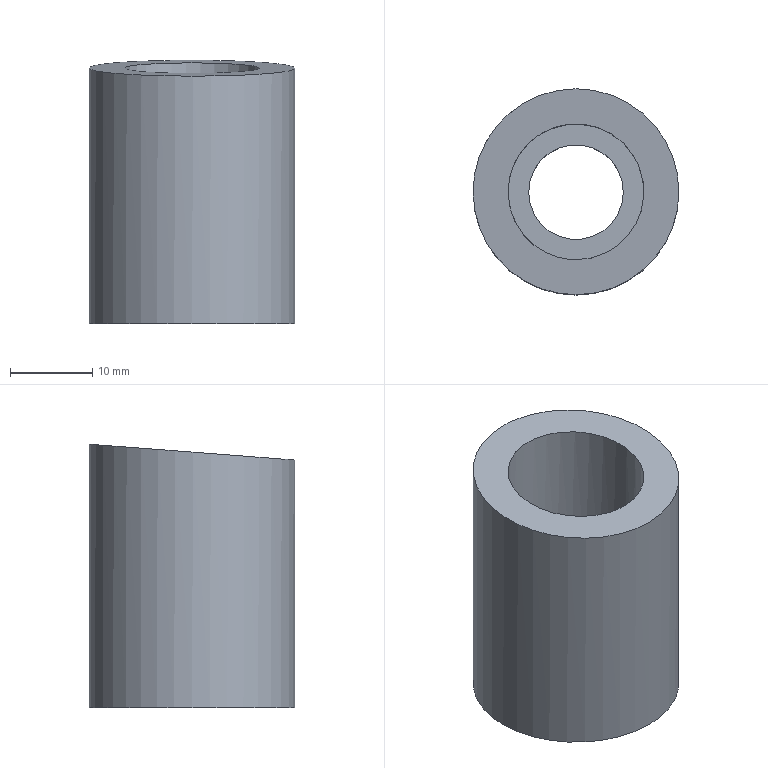Part | NX | features solid 2 | 1 solid | 6 faces | box 25 x 25 x 32.007 mm | volume 9815 mm3 | plane 3 | cylinder 3 | commonest cylinder face diameters 11.5 x1 16.5 x1 25 x1
STEP:
#1=CARTESIAN_POINT('',(-503.5,9.,-58.));
#2=VERTEX_POINT('',#1);
#3=CARTESIAN_POINT('',(-516.,9.,-58.));
#4=DIRECTION('',(0.,0.,1.));
#5=DIRECTION('',(1.,0.,0.));
#6=AXIS2_PLACEMENT_3D('',#3,#4,#5);
#7=CIRCLE('',#6,12.5);
#8=EDGE_CURVE('',#2,#2,#7,.T.);
#9=ORIENTED_EDGE('',*,*,#8,.F.);
#10=EDGE_LOOP('',(#9));
#11=FACE_BOUND('',#10,.T.);
#12=CARTESIAN_POINT('',(-510.25,9.,-58.));
#13=VERTEX_POINT('',#12);
#14=CARTESIAN_POINT('',(-516.,9.,-58.));
#15=DIRECTION('',(0.,0.,1.));
#16=DIRECTION('',(1.,0.,0.));
#17=AXIS2_PLACEMENT_3D('',#14,#15,#16);
#18=CIRCLE('',#17,5.75);
#19=EDGE_CURVE('',#13,#13,#18,.F.);
#20=ORIENTED_EDGE('',*,*,#19,.F.);
#21=EDGE_LOOP('',(#20));
#22=FACE_BOUND('',#21,.T.);
#23=CARTESIAN_POINT('',(-516.,9.,-58.));
#24=DIRECTION('',(0.,0.,1.));
#25=DIRECTION('',(1.,0.,0.));
#26=AXIS2_PLACEMENT_3D('',#23,#24,#25);
#27=PLANE('',#26);
#28=ADVANCED_FACE('',(#11,#22),#27,.F.);
#29=CARTESIAN_POINT('',(-507.75,9.,-46.955));
#30=VERTEX_POINT('',#29);
#31=CARTESIAN_POINT('',(-516.,9.,-46.955));
#32=DIRECTION('',(0.,0.,1.));
#33=DIRECTION('',(1.,0.,0.));
#34=AXIS2_PLACEMENT_3D('',#31,#32,#33);
#35=CIRCLE('',#34,8.25);
#36=EDGE_CURVE('',#30,#30,#35,.T.);
#37=ORIENTED_EDGE('',*,*,#36,.T.);
#38=EDGE_LOOP('',(#37));
#39=FACE_BOUND('',#38,.T.);
#40=CARTESIAN_POINT('',(-510.25,9.,-46.955));
#41=VERTEX_POINT('',#40);
#42=CARTESIAN_POINT('',(-516.,9.,-46.955));
#43=DIRECTION('',(0.,0.,1.));
#44=DIRECTION('',(1.,0.,0.));
#45=AXIS2_PLACEMENT_3D('',#42,#43,#44);
#46=CIRCLE('',#45,5.75);
#47=EDGE_CURVE('',#41,#41,#46,.F.);
#48=ORIENTED_EDGE('',*,*,#47,.T.);
#49=EDGE_LOOP('',(#48));
#50=FACE_BOUND('',#49,.T.);
#51=CARTESIAN_POINT('',(-516.,9.,-46.955));
#52=DIRECTION('',(0.,0.,1.));
#53=DIRECTION('',(1.,0.,0.));
#54=AXIS2_PLACEMENT_3D('',#51,#52,#53);
#55=PLANE('',#54);
#56=ADVANCED_FACE('',(#39,#50),#55,.T.);
#57=CARTESIAN_POINT('',(-516.124,21.499,-25.993));
#58=VERTEX_POINT('',#57);
#59=CARTESIAN_POINT('',(-516.,9.,-26.955));
#60=DIRECTION('',(0.0007587,-0.07675,0.9971));
#61=DIRECTION('',(-0.009856,0.997,0.07675));
#62=AXIS2_PLACEMENT_3D('',#59,#60,#61);
#63=ELLIPSE('',#62,12.537,12.5);
#64=EDGE_CURVE('',#58,#58,#63,.T.);
#65=ORIENTED_EDGE('',*,*,#64,.T.);
#66=EDGE_LOOP('',(#65));
#67=FACE_BOUND('',#66,.T.);
#68=CARTESIAN_POINT('',(-515.918,0.7504,-27.59));
#69=VERTEX_POINT('',#68);
#70=CARTESIAN_POINT('',(-516.,9.,-26.955));
#71=DIRECTION('',(0.0007587,-0.07675,0.9971));
#72=DIRECTION('',(0.009856,-0.997,-0.07675));
#73=AXIS2_PLACEMENT_3D('',#70,#71,#72);
#74=ELLIPSE('',#73,8.274,8.25);
#75=EDGE_CURVE('',#69,#69,#74,.F.);
#76=ORIENTED_EDGE('',*,*,#75,.T.);
#77=EDGE_LOOP('',(#76));
#78=FACE_BOUND('',#77,.T.);
#79=CARTESIAN_POINT('',(-530.071,161.723,-15.189));
#80=DIRECTION('',(0.0007587,-0.07675,0.9971));
#81=DIRECTION('',(-1.,0.004401,0.0011));
#82=AXIS2_PLACEMENT_3D('',#79,#80,#81);
#83=PLANE('',#82);
#84=ADVANCED_FACE('',(#67,#78),#83,.T.);
#85=ORIENTED_EDGE('',*,*,#8,.T.);
#86=EDGE_LOOP('',(#85));
#87=FACE_BOUND('',#86,.T.);
#88=ORIENTED_EDGE('',*,*,#64,.F.);
#89=EDGE_LOOP('',(#88));
#90=FACE_BOUND('',#89,.T.);
#91=CARTESIAN_POINT('',(-516.,9.,-58.));
#92=DIRECTION('',(0.,0.,1.));
#93=DIRECTION('',(1.,0.,0.));
#94=AXIS2_PLACEMENT_3D('',#91,#92,#93);
#95=CYLINDRICAL_SURFACE('',#94,12.5);
#96=ADVANCED_FACE('',(#87,#90),#95,.T.);
#97=ORIENTED_EDGE('',*,*,#75,.F.);
#98=EDGE_LOOP('',(#97));
#99=FACE_BOUND('',#98,.T.);
#100=ORIENTED_EDGE('',*,*,#36,.F.);
#101=EDGE_LOOP('',(#100));
#102=FACE_BOUND('',#101,.T.);
#103=CARTESIAN_POINT('',(-516.,9.,-16.955));
#104=DIRECTION('',(0.,0.,-1.));
#105=DIRECTION('',(-1.,0.,0.));
#106=AXIS2_PLACEMENT_3D('',#103,#104,#105);
#107=CYLINDRICAL_SURFACE('',#106,8.25);
#108=ADVANCED_FACE('',(#99,#102),#107,.F.);
#109=ORIENTED_EDGE('',*,*,#47,.F.);
#110=EDGE_LOOP('',(#109));
#111=FACE_BOUND('',#110,.T.);
#112=ORIENTED_EDGE('',*,*,#19,.T.);
#113=EDGE_LOOP('',(#112));
#114=FACE_BOUND('',#113,.T.);
#115=CARTESIAN_POINT('',(-516.,9.,73.045));
#116=DIRECTION('',(0.,0.,-1.));
#117=DIRECTION('',(-1.,0.,0.));
#118=AXIS2_PLACEMENT_3D('',#115,#116,#117);
#119=CYLINDRICAL_SURFACE('',#118,5.75);
#120=ADVANCED_FACE('',(#111,#114),#119,.F.);
#121=CLOSED_SHELL('',(#28,#56,#84,#96,#108,#120));
#122=MANIFOLD_SOLID_BREP('',#121);
#123=(LENGTH_UNIT()NAMED_UNIT(*)SI_UNIT(.MILLI.,.METRE.));
#124=UNCERTAINTY_MEASURE_WITH_UNIT(LENGTH_MEASURE(0.00001),#123,'','');
#125=(NAMED_UNIT(*)PLANE_ANGLE_UNIT()SI_UNIT($,.RADIAN.));
#126=(NAMED_UNIT(*)SI_UNIT($,.STERADIAN.)SOLID_ANGLE_UNIT());
#127=(GEOMETRIC_REPRESENTATION_CONTEXT(3)GLOBAL_UNCERTAINTY_ASSIGNED_CONTEXT((#124))GLOBAL_UNIT_ASSIGNED_CONTEXT((#123,#125,#126))REPRESENTATION_CONTEXT('',''));
#128=ADVANCED_BREP_SHAPE_REPRESENTATION('',(#122),#127);